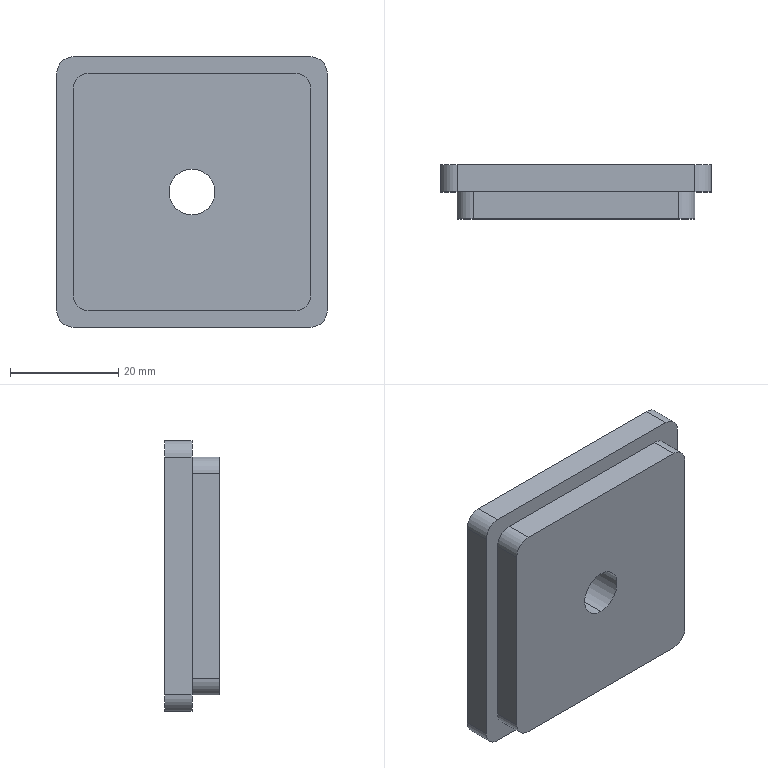Part | STEP file | Microwave Drying Flat Conveyor-CN2500x400-105-105 | 1 solid | 21 faces | box 50 x 10 x 50 mm | volume 21535 mm3 | plane 11 | cylinder 10 | commonest cylinder face diameters 6 x8 8.5 x2
STEP:
#1=CARTESIAN_POINT('',(0.,0.,-4.25));
#2=VERTEX_POINT('',#1);
#3=CARTESIAN_POINT('',(0.,0.,4.25));
#4=VERTEX_POINT('',#3);
#5=CARTESIAN_POINT('',(0.,0.,0.));
#6=DIRECTION('',(0.,1.,0.));
#7=DIRECTION('',(0.,0.,1.));
#8=AXIS2_PLACEMENT_3D('',#5,#6,#7);
#9=CIRCLE('',#8,4.25);
#10=EDGE_CURVE('',#2,#4,#9,.T.);
#11=ORIENTED_EDGE('',*,*,#10,.F.);
#12=CARTESIAN_POINT('',(0.,10.,-4.25));
#13=VERTEX_POINT('',#12);
#14=CARTESIAN_POINT('',(0.,10.,-4.25));
#15=DIRECTION('',(0.,1.,0.));
#16=VECTOR('',#15,1000.);
#17=LINE('',#14,#16);
#18=EDGE_CURVE('',#2,#13,#17,.T.);
#19=ORIENTED_EDGE('',*,*,#18,.T.);
#20=CARTESIAN_POINT('',(0.,10.,4.25));
#21=VERTEX_POINT('',#20);
#22=CARTESIAN_POINT('',(0.,10.,0.));
#23=DIRECTION('',(0.,1.,0.));
#24=DIRECTION('',(0.,0.,1.));
#25=AXIS2_PLACEMENT_3D('',#22,#23,#24);
#26=CIRCLE('',#25,4.25);
#27=EDGE_CURVE('',#13,#21,#26,.T.);
#28=ORIENTED_EDGE('',*,*,#27,.T.);
#29=CARTESIAN_POINT('',(0.,10.,4.25));
#30=DIRECTION('',(0.,1.,0.));
#31=VECTOR('',#30,1000.);
#32=LINE('',#29,#31);
#33=EDGE_CURVE('',#4,#21,#32,.T.);
#34=ORIENTED_EDGE('',*,*,#33,.F.);
#35=EDGE_LOOP('',(#11,#19,#28,#34));
#36=FACE_OUTER_BOUND('',#35,.T.);
#37=CARTESIAN_POINT('',(0.,10.,0.));
#38=DIRECTION('',(0.,1.,0.));
#39=DIRECTION('',(0.,0.,1.));
#40=AXIS2_PLACEMENT_3D('',#37,#38,#39);
#41=CYLINDRICAL_SURFACE('',#40,4.25);
#42=ADVANCED_FACE('',(#36),#41,.F.);
#43=CARTESIAN_POINT('',(25.,5.,22.));
#44=VERTEX_POINT('',#43);
#45=CARTESIAN_POINT('',(22.,5.,25.));
#46=VERTEX_POINT('',#45);
#47=CARTESIAN_POINT('',(22.,5.,22.));
#48=DIRECTION('',(0.,-1.,0.));
#49=DIRECTION('',(0.,0.,-1.));
#50=AXIS2_PLACEMENT_3D('',#47,#48,#49);
#51=CIRCLE('',#50,3.);
#52=EDGE_CURVE('',#44,#46,#51,.T.);
#53=ORIENTED_EDGE('',*,*,#52,.F.);
#54=CARTESIAN_POINT('',(25.,10.,22.));
#55=VERTEX_POINT('',#54);
#56=CARTESIAN_POINT('',(25.,10.,22.));
#57=DIRECTION('',(0.,-1.,0.));
#58=VECTOR('',#57,1000.);
#59=LINE('',#56,#58);
#60=EDGE_CURVE('',#55,#44,#59,.T.);
#61=ORIENTED_EDGE('',*,*,#60,.F.);
#62=CARTESIAN_POINT('',(22.,10.,25.));
#63=VERTEX_POINT('',#62);
#64=CARTESIAN_POINT('',(22.,10.,22.));
#65=DIRECTION('',(0.,1.,0.));
#66=DIRECTION('',(0.,0.,1.));
#67=AXIS2_PLACEMENT_3D('',#64,#65,#66);
#68=CIRCLE('',#67,3.);
#69=EDGE_CURVE('',#63,#55,#68,.T.);
#70=ORIENTED_EDGE('',*,*,#69,.F.);
#71=CARTESIAN_POINT('',(22.,10.,25.));
#72=DIRECTION('',(0.,-1.,0.));
#73=VECTOR('',#72,1000.);
#74=LINE('',#71,#73);
#75=EDGE_CURVE('',#63,#46,#74,.T.);
#76=ORIENTED_EDGE('',*,*,#75,.T.);
#77=EDGE_LOOP('',(#53,#61,#70,#76));
#78=FACE_OUTER_BOUND('',#77,.T.);
#79=CARTESIAN_POINT('',(22.,10.,22.));
#80=DIRECTION('',(0.,-1.,0.));
#81=DIRECTION('',(0.,0.,-1.));
#82=AXIS2_PLACEMENT_3D('',#79,#80,#81);
#83=CYLINDRICAL_SURFACE('',#82,3.);
#84=ADVANCED_FACE('',(#78),#83,.T.);
#85=CARTESIAN_POINT('',(25.,5.,-22.));
#86=VERTEX_POINT('',#85);
#87=CARTESIAN_POINT('',(25.,5.,22.));
#88=DIRECTION('',(0.,0.,1.));
#89=VECTOR('',#88,1000.);
#90=LINE('',#87,#89);
#91=EDGE_CURVE('',#86,#44,#90,.T.);
#92=ORIENTED_EDGE('',*,*,#91,.F.);
#93=CARTESIAN_POINT('',(25.,10.,-22.));
#94=VERTEX_POINT('',#93);
#95=CARTESIAN_POINT('',(25.,10.,-22.));
#96=DIRECTION('',(0.,-1.,0.));
#97=VECTOR('',#96,1000.);
#98=LINE('',#95,#97);
#99=EDGE_CURVE('',#94,#86,#98,.T.);
#100=ORIENTED_EDGE('',*,*,#99,.F.);
#101=CARTESIAN_POINT('',(25.,10.,-22.));
#102=DIRECTION('',(0.,0.,-1.));
#103=VECTOR('',#102,1000.);
#104=LINE('',#101,#103);
#105=EDGE_CURVE('',#55,#94,#104,.T.);
#106=ORIENTED_EDGE('',*,*,#105,.F.);
#107=ORIENTED_EDGE('',*,*,#60,.T.);
#108=EDGE_LOOP('',(#92,#100,#106,#107));
#109=FACE_OUTER_BOUND('',#108,.T.);
#110=CARTESIAN_POINT('',(25.,10.,-22.));
#111=DIRECTION('',(-1.,0.,0.));
#112=DIRECTION('',(0.,0.,1.));
#113=AXIS2_PLACEMENT_3D('',#110,#111,#112);
#114=PLANE('',#113);
#115=ADVANCED_FACE('',(#109),#114,.F.);
#116=CARTESIAN_POINT('',(22.,5.,-25.));
#117=VERTEX_POINT('',#116);
#118=CARTESIAN_POINT('',(22.,5.,-22.));
#119=DIRECTION('',(0.,-1.,0.));
#120=DIRECTION('',(0.,0.,-1.));
#121=AXIS2_PLACEMENT_3D('',#118,#119,#120);
#122=CIRCLE('',#121,3.);
#123=EDGE_CURVE('',#117,#86,#122,.T.);
#124=ORIENTED_EDGE('',*,*,#123,.F.);
#125=CARTESIAN_POINT('',(22.,10.,-25.));
#126=VERTEX_POINT('',#125);
#127=CARTESIAN_POINT('',(22.,10.,-25.));
#128=DIRECTION('',(0.,-1.,0.));
#129=VECTOR('',#128,1000.);
#130=LINE('',#127,#129);
#131=EDGE_CURVE('',#126,#117,#130,.T.);
#132=ORIENTED_EDGE('',*,*,#131,.F.);
#133=CARTESIAN_POINT('',(22.,10.,-22.));
#134=DIRECTION('',(0.,1.,0.));
#135=DIRECTION('',(0.,0.,-1.));
#136=AXIS2_PLACEMENT_3D('',#133,#134,#135);
#137=CIRCLE('',#136,3.);
#138=EDGE_CURVE('',#94,#126,#137,.T.);
#139=ORIENTED_EDGE('',*,*,#138,.F.);
#140=ORIENTED_EDGE('',*,*,#99,.T.);
#141=EDGE_LOOP('',(#124,#132,#139,#140));
#142=FACE_OUTER_BOUND('',#141,.T.);
#143=CARTESIAN_POINT('',(22.,10.,-22.));
#144=DIRECTION('',(0.,-1.,0.));
#145=DIRECTION('',(0.,0.,-1.));
#146=AXIS2_PLACEMENT_3D('',#143,#144,#145);
#147=CYLINDRICAL_SURFACE('',#146,3.);
#148=ADVANCED_FACE('',(#142),#147,.T.);
#149=CARTESIAN_POINT('',(-22.,5.,-25.));
#150=VERTEX_POINT('',#149);
#151=CARTESIAN_POINT('',(22.,5.,-25.));
#152=DIRECTION('',(1.,0.,0.));
#153=VECTOR('',#152,1000.);
#154=LINE('',#151,#153);
#155=EDGE_CURVE('',#150,#117,#154,.T.);
#156=ORIENTED_EDGE('',*,*,#155,.F.);
#157=CARTESIAN_POINT('',(-22.,10.,-25.));
#158=VERTEX_POINT('',#157);
#159=CARTESIAN_POINT('',(-22.,10.,-25.));
#160=DIRECTION('',(0.,-1.,0.));
#161=VECTOR('',#160,1000.);
#162=LINE('',#159,#161);
#163=EDGE_CURVE('',#158,#150,#162,.T.);
#164=ORIENTED_EDGE('',*,*,#163,.F.);
#165=CARTESIAN_POINT('',(-22.,10.,-25.));
#166=DIRECTION('',(-1.,0.,0.));
#167=VECTOR('',#166,1000.);
#168=LINE('',#165,#167);
#169=EDGE_CURVE('',#126,#158,#168,.T.);
#170=ORIENTED_EDGE('',*,*,#169,.F.);
#171=ORIENTED_EDGE('',*,*,#131,.T.);
#172=EDGE_LOOP('',(#156,#164,#170,#171));
#173=FACE_OUTER_BOUND('',#172,.T.);
#174=CARTESIAN_POINT('',(-22.,10.,-25.));
#175=DIRECTION('',(0.,0.,1.));
#176=DIRECTION('',(1.,0.,0.));
#177=AXIS2_PLACEMENT_3D('',#174,#175,#176);
#178=PLANE('',#177);
#179=ADVANCED_FACE('',(#173),#178,.F.);
#180=CARTESIAN_POINT('',(-25.,5.,-22.));
#181=VERTEX_POINT('',#180);
#182=CARTESIAN_POINT('',(-22.,5.,-22.));
#183=DIRECTION('',(0.,-1.,0.));
#184=DIRECTION('',(0.,0.,-1.));
#185=AXIS2_PLACEMENT_3D('',#182,#183,#184);
#186=CIRCLE('',#185,3.);
#187=EDGE_CURVE('',#181,#150,#186,.T.);
#188=ORIENTED_EDGE('',*,*,#187,.F.);
#189=CARTESIAN_POINT('',(-25.,10.,-22.));
#190=VERTEX_POINT('',#189);
#191=CARTESIAN_POINT('',(-25.,10.,-22.));
#192=DIRECTION('',(0.,-1.,0.));
#193=VECTOR('',#192,1000.);
#194=LINE('',#191,#193);
#195=EDGE_CURVE('',#190,#181,#194,.T.);
#196=ORIENTED_EDGE('',*,*,#195,.F.);
#197=CARTESIAN_POINT('',(-22.,10.,-22.));
#198=DIRECTION('',(0.,1.,0.));
#199=DIRECTION('',(0.,0.,1.));
#200=AXIS2_PLACEMENT_3D('',#197,#198,#199);
#201=CIRCLE('',#200,3.);
#202=EDGE_CURVE('',#158,#190,#201,.T.);
#203=ORIENTED_EDGE('',*,*,#202,.F.);
#204=ORIENTED_EDGE('',*,*,#163,.T.);
#205=EDGE_LOOP('',(#188,#196,#203,#204));
#206=FACE_OUTER_BOUND('',#205,.T.);
#207=CARTESIAN_POINT('',(-22.,10.,-22.));
#208=DIRECTION('',(0.,-1.,0.));
#209=DIRECTION('',(0.,0.,-1.));
#210=AXIS2_PLACEMENT_3D('',#207,#208,#209);
#211=CYLINDRICAL_SURFACE('',#210,3.);
#212=ADVANCED_FACE('',(#206),#211,.T.);
#213=CARTESIAN_POINT('',(-25.,5.,22.));
#214=VERTEX_POINT('',#213);
#215=CARTESIAN_POINT('',(-25.,5.,-22.));
#216=DIRECTION('',(0.,0.,-1.));
#217=VECTOR('',#216,1000.);
#218=LINE('',#215,#217);
#219=EDGE_CURVE('',#214,#181,#218,.T.);
#220=ORIENTED_EDGE('',*,*,#219,.F.);
#221=CARTESIAN_POINT('',(-25.,10.,22.));
#222=VERTEX_POINT('',#221);
#223=CARTESIAN_POINT('',(-25.,10.,22.));
#224=DIRECTION('',(0.,-1.,0.));
#225=VECTOR('',#224,1000.);
#226=LINE('',#223,#225);
#227=EDGE_CURVE('',#222,#214,#226,.T.);
#228=ORIENTED_EDGE('',*,*,#227,.F.);
#229=CARTESIAN_POINT('',(-25.,10.,-22.));
#230=DIRECTION('',(0.,0.,1.));
#231=VECTOR('',#230,1000.);
#232=LINE('',#229,#231);
#233=EDGE_CURVE('',#190,#222,#232,.T.);
#234=ORIENTED_EDGE('',*,*,#233,.F.);
#235=ORIENTED_EDGE('',*,*,#195,.T.);
#236=EDGE_LOOP('',(#220,#228,#234,#235));
#237=FACE_OUTER_BOUND('',#236,.T.);
#238=CARTESIAN_POINT('',(-25.,10.,-22.));
#239=DIRECTION('',(1.,0.,0.));
#240=DIRECTION('',(0.,0.,-1.));
#241=AXIS2_PLACEMENT_3D('',#238,#239,#240);
#242=PLANE('',#241);
#243=ADVANCED_FACE('',(#237),#242,.F.);
#244=CARTESIAN_POINT('',(-22.,5.,25.));
#245=VERTEX_POINT('',#244);
#246=CARTESIAN_POINT('',(-22.,5.,22.));
#247=DIRECTION('',(0.,-1.,0.));
#248=DIRECTION('',(0.,0.,-1.));
#249=AXIS2_PLACEMENT_3D('',#246,#247,#248);
#250=CIRCLE('',#249,3.);
#251=EDGE_CURVE('',#245,#214,#250,.T.);
#252=ORIENTED_EDGE('',*,*,#251,.F.);
#253=CARTESIAN_POINT('',(-22.,10.,25.));
#254=VERTEX_POINT('',#253);
#255=CARTESIAN_POINT('',(-22.,10.,25.));
#256=DIRECTION('',(0.,-1.,0.));
#257=VECTOR('',#256,1000.);
#258=LINE('',#255,#257);
#259=EDGE_CURVE('',#254,#245,#258,.T.);
#260=ORIENTED_EDGE('',*,*,#259,.F.);
#261=CARTESIAN_POINT('',(-22.,10.,22.));
#262=DIRECTION('',(0.,1.,0.));
#263=DIRECTION('',(0.,0.,1.));
#264=AXIS2_PLACEMENT_3D('',#261,#262,#263);
#265=CIRCLE('',#264,3.);
#266=EDGE_CURVE('',#222,#254,#265,.T.);
#267=ORIENTED_EDGE('',*,*,#266,.F.);
#268=ORIENTED_EDGE('',*,*,#227,.T.);
#269=EDGE_LOOP('',(#252,#260,#267,#268));
#270=FACE_OUTER_BOUND('',#269,.T.);
#271=CARTESIAN_POINT('',(-22.,10.,22.));
#272=DIRECTION('',(0.,-1.,0.));
#273=DIRECTION('',(0.,0.,-1.));
#274=AXIS2_PLACEMENT_3D('',#271,#272,#273);
#275=CYLINDRICAL_SURFACE('',#274,3.);
#276=ADVANCED_FACE('',(#270),#275,.T.);
#277=CARTESIAN_POINT('',(-22.,5.,25.));
#278=DIRECTION('',(-1.,0.,0.));
#279=VECTOR('',#278,1000.);
#280=LINE('',#277,#279);
#281=EDGE_CURVE('',#46,#245,#280,.T.);
#282=ORIENTED_EDGE('',*,*,#281,.F.);
#283=ORIENTED_EDGE('',*,*,#75,.F.);
#284=CARTESIAN_POINT('',(-22.,10.,25.));
#285=DIRECTION('',(1.,0.,0.));
#286=VECTOR('',#285,1000.);
#287=LINE('',#284,#286);
#288=EDGE_CURVE('',#254,#63,#287,.T.);
#289=ORIENTED_EDGE('',*,*,#288,.F.);
#290=ORIENTED_EDGE('',*,*,#259,.T.);
#291=EDGE_LOOP('',(#282,#283,#289,#290));
#292=FACE_OUTER_BOUND('',#291,.T.);
#293=CARTESIAN_POINT('',(-22.,10.,25.));
#294=DIRECTION('',(0.,0.,-1.));
#295=DIRECTION('',(-1.,0.,0.));
#296=AXIS2_PLACEMENT_3D('',#293,#294,#295);
#297=PLANE('',#296);
#298=ADVANCED_FACE('',(#292),#297,.F.);
#299=CARTESIAN_POINT('',(0.,0.,0.));
#300=DIRECTION('',(0.,1.,0.));
#301=DIRECTION('',(0.,0.,1.));
#302=AXIS2_PLACEMENT_3D('',#299,#300,#301);
#303=CIRCLE('',#302,4.25);
#304=EDGE_CURVE('',#4,#2,#303,.T.);
#305=ORIENTED_EDGE('',*,*,#304,.T.);
#306=ORIENTED_EDGE('',*,*,#10,.T.);
#307=EDGE_LOOP('',(#305,#306));
#308=FACE_BOUND('',#307,.T.);
#309=CARTESIAN_POINT('',(-22.,0.,19.));
#310=VERTEX_POINT('',#309);
#311=CARTESIAN_POINT('',(-22.,0.,-19.));
#312=VERTEX_POINT('',#311);
#313=CARTESIAN_POINT('',(-22.,0.,22.));
#314=DIRECTION('',(0.,0.,-1.));
#315=VECTOR('',#314,1000.);
#316=LINE('',#313,#315);
#317=EDGE_CURVE('',#310,#312,#316,.T.);
#318=ORIENTED_EDGE('',*,*,#317,.T.);
#319=CARTESIAN_POINT('',(-19.,0.,-22.));
#320=VERTEX_POINT('',#319);
#321=CARTESIAN_POINT('',(-19.,0.,-19.));
#322=DIRECTION('',(0.,-1.,0.));
#323=DIRECTION('',(0.,0.,1.));
#324=AXIS2_PLACEMENT_3D('',#321,#322,#323);
#325=CIRCLE('',#324,3.);
#326=EDGE_CURVE('',#312,#320,#325,.T.);
#327=ORIENTED_EDGE('',*,*,#326,.T.);
#328=CARTESIAN_POINT('',(19.,0.,-22.));
#329=VERTEX_POINT('',#328);
#330=CARTESIAN_POINT('',(-22.,0.,-22.));
#331=DIRECTION('',(1.,0.,0.));
#332=VECTOR('',#331,1000.);
#333=LINE('',#330,#332);
#334=EDGE_CURVE('',#320,#329,#333,.T.);
#335=ORIENTED_EDGE('',*,*,#334,.T.);
#336=CARTESIAN_POINT('',(22.,0.,-19.));
#337=VERTEX_POINT('',#336);
#338=CARTESIAN_POINT('',(19.,0.,-19.));
#339=DIRECTION('',(0.,-1.,0.));
#340=DIRECTION('',(0.,0.,1.));
#341=AXIS2_PLACEMENT_3D('',#338,#339,#340);
#342=CIRCLE('',#341,3.);
#343=EDGE_CURVE('',#329,#337,#342,.T.);
#344=ORIENTED_EDGE('',*,*,#343,.T.);
#345=CARTESIAN_POINT('',(22.,0.,19.));
#346=VERTEX_POINT('',#345);
#347=CARTESIAN_POINT('',(22.,0.,-22.));
#348=DIRECTION('',(0.,0.,1.));
#349=VECTOR('',#348,1000.);
#350=LINE('',#347,#349);
#351=EDGE_CURVE('',#337,#346,#350,.T.);
#352=ORIENTED_EDGE('',*,*,#351,.T.);
#353=CARTESIAN_POINT('',(19.,0.,22.));
#354=VERTEX_POINT('',#353);
#355=CARTESIAN_POINT('',(19.,0.,19.));
#356=DIRECTION('',(0.,-1.,0.));
#357=DIRECTION('',(0.,0.,1.));
#358=AXIS2_PLACEMENT_3D('',#355,#356,#357);
#359=CIRCLE('',#358,3.);
#360=EDGE_CURVE('',#346,#354,#359,.T.);
#361=ORIENTED_EDGE('',*,*,#360,.T.);
#362=CARTESIAN_POINT('',(-19.,0.,22.));
#363=VERTEX_POINT('',#362);
#364=CARTESIAN_POINT('',(22.,0.,22.));
#365=DIRECTION('',(-1.,0.,0.));
#366=VECTOR('',#365,1000.);
#367=LINE('',#364,#366);
#368=EDGE_CURVE('',#354,#363,#367,.T.);
#369=ORIENTED_EDGE('',*,*,#368,.T.);
#370=CARTESIAN_POINT('',(-19.,0.,19.));
#371=DIRECTION('',(0.,-1.,0.));
#372=DIRECTION('',(0.,0.,1.));
#373=AXIS2_PLACEMENT_3D('',#370,#371,#372);
#374=CIRCLE('',#373,3.);
#375=EDGE_CURVE('',#363,#310,#374,.T.);
#376=ORIENTED_EDGE('',*,*,#375,.T.);
#377=EDGE_LOOP('',(#318,#327,#335,#344,#352,#361,#369,#376));
#378=FACE_OUTER_BOUND('',#377,.T.);
#379=CARTESIAN_POINT('',(22.,0.,22.));
#380=DIRECTION('',(0.,1.,0.));
#381=DIRECTION('',(0.,0.,1.));
#382=AXIS2_PLACEMENT_3D('',#379,#380,#381);
#383=PLANE('',#382);
#384=ADVANCED_FACE('',(#308,#378),#383,.F.);
#385=CARTESIAN_POINT('',(0.,10.,0.));
#386=DIRECTION('',(0.,1.,0.));
#387=DIRECTION('',(0.,0.,1.));
#388=AXIS2_PLACEMENT_3D('',#385,#386,#387);
#389=CIRCLE('',#388,4.25);
#390=EDGE_CURVE('',#21,#13,#389,.T.);
#391=ORIENTED_EDGE('',*,*,#390,.F.);
#392=ORIENTED_EDGE('',*,*,#27,.F.);
#393=EDGE_LOOP('',(#391,#392));
#394=FACE_BOUND('',#393,.T.);
#395=ORIENTED_EDGE('',*,*,#69,.T.);
#396=ORIENTED_EDGE('',*,*,#105,.T.);
#397=ORIENTED_EDGE('',*,*,#138,.T.);
#398=ORIENTED_EDGE('',*,*,#169,.T.);
#399=ORIENTED_EDGE('',*,*,#202,.T.);
#400=ORIENTED_EDGE('',*,*,#233,.T.);
#401=ORIENTED_EDGE('',*,*,#266,.T.);
#402=ORIENTED_EDGE('',*,*,#288,.T.);
#403=EDGE_LOOP('',(#395,#396,#397,#398,#399,#400,#401,#402));
#404=FACE_OUTER_BOUND('',#403,.T.);
#405=CARTESIAN_POINT('',(22.,10.,22.));
#406=DIRECTION('',(0.,1.,0.));
#407=DIRECTION('',(0.,0.,1.));
#408=AXIS2_PLACEMENT_3D('',#405,#406,#407);
#409=PLANE('',#408);
#410=ADVANCED_FACE('',(#394,#404),#409,.T.);
#411=ORIENTED_EDGE('',*,*,#18,.F.);
#412=ORIENTED_EDGE('',*,*,#304,.F.);
#413=ORIENTED_EDGE('',*,*,#33,.T.);
#414=ORIENTED_EDGE('',*,*,#390,.T.);
#415=EDGE_LOOP('',(#411,#412,#413,#414));
#416=FACE_OUTER_BOUND('',#415,.T.);
#417=CARTESIAN_POINT('',(0.,10.,0.));
#418=DIRECTION('',(0.,1.,0.));
#419=DIRECTION('',(0.,0.,1.));
#420=AXIS2_PLACEMENT_3D('',#417,#418,#419);
#421=CYLINDRICAL_SURFACE('',#420,4.25);
#422=ADVANCED_FACE('',(#416),#421,.F.);
#423=CARTESIAN_POINT('',(-19.,5.,-22.));
#424=VERTEX_POINT('',#423);
#425=CARTESIAN_POINT('',(19.,5.,-22.));
#426=VERTEX_POINT('',#425);
#427=CARTESIAN_POINT('',(-22.,5.,-22.));
#428=DIRECTION('',(1.,0.,0.));
#429=VECTOR('',#428,1000.);
#430=LINE('',#427,#429);
#431=EDGE_CURVE('',#424,#426,#430,.T.);
#432=ORIENTED_EDGE('',*,*,#431,.F.);
#433=CARTESIAN_POINT('',(-22.,5.,-19.));
#434=VERTEX_POINT('',#433);
#435=CARTESIAN_POINT('',(-19.,5.,-19.));
#436=DIRECTION('',(0.,1.,0.));
#437=DIRECTION('',(0.,0.,-1.));
#438=AXIS2_PLACEMENT_3D('',#435,#436,#437);
#439=CIRCLE('',#438,3.);
#440=EDGE_CURVE('',#424,#434,#439,.T.);
#441=ORIENTED_EDGE('',*,*,#440,.T.);
#442=CARTESIAN_POINT('',(-22.,5.,19.));
#443=VERTEX_POINT('',#442);
#444=CARTESIAN_POINT('',(-22.,5.,22.));
#445=DIRECTION('',(0.,0.,-1.));
#446=VECTOR('',#445,1000.);
#447=LINE('',#444,#446);
#448=EDGE_CURVE('',#443,#434,#447,.T.);
#449=ORIENTED_EDGE('',*,*,#448,.F.);
#450=CARTESIAN_POINT('',(-19.,5.,22.));
#451=VERTEX_POINT('',#450);
#452=CARTESIAN_POINT('',(-19.,5.,19.));
#453=DIRECTION('',(0.,1.,0.));
#454=DIRECTION('',(0.,0.,-1.));
#455=AXIS2_PLACEMENT_3D('',#452,#453,#454);
#456=CIRCLE('',#455,3.);
#457=EDGE_CURVE('',#443,#451,#456,.T.);
#458=ORIENTED_EDGE('',*,*,#457,.T.);
#459=CARTESIAN_POINT('',(19.,5.,22.));
#460=VERTEX_POINT('',#459);
#461=CARTESIAN_POINT('',(22.,5.,22.));
#462=DIRECTION('',(-1.,0.,0.));
#463=VECTOR('',#462,1000.);
#464=LINE('',#461,#463);
#465=EDGE_CURVE('',#460,#451,#464,.T.);
#466=ORIENTED_EDGE('',*,*,#465,.F.);
#467=CARTESIAN_POINT('',(22.,5.,19.));
#468=VERTEX_POINT('',#467);
#469=CARTESIAN_POINT('',(19.,5.,19.));
#470=DIRECTION('',(0.,1.,0.));
#471=DIRECTION('',(0.,0.,-1.));
#472=AXIS2_PLACEMENT_3D('',#469,#470,#471);
#473=CIRCLE('',#472,3.);
#474=EDGE_CURVE('',#460,#468,#473,.T.);
#475=ORIENTED_EDGE('',*,*,#474,.T.);
#476=CARTESIAN_POINT('',(22.,5.,-19.));
#477=VERTEX_POINT('',#476);
#478=CARTESIAN_POINT('',(22.,5.,-22.));
#479=DIRECTION('',(0.,0.,1.));
#480=VECTOR('',#479,1000.);
#481=LINE('',#478,#480);
#482=EDGE_CURVE('',#477,#468,#481,.T.);
#483=ORIENTED_EDGE('',*,*,#482,.F.);
#484=CARTESIAN_POINT('',(19.,5.,-19.));
#485=DIRECTION('',(0.,1.,0.));
#486=DIRECTION('',(0.,0.,-1.));
#487=AXIS2_PLACEMENT_3D('',#484,#485,#486);
#488=CIRCLE('',#487,3.);
#489=EDGE_CURVE('',#477,#426,#488,.T.);
#490=ORIENTED_EDGE('',*,*,#489,.T.);
#491=EDGE_LOOP('',(#432,#441,#449,#458,#466,#475,#483,#490));
#492=FACE_BOUND('',#491,.T.);
#493=ORIENTED_EDGE('',*,*,#251,.T.);
#494=ORIENTED_EDGE('',*,*,#219,.T.);
#495=ORIENTED_EDGE('',*,*,#187,.T.);
#496=ORIENTED_EDGE('',*,*,#155,.T.);
#497=ORIENTED_EDGE('',*,*,#123,.T.);
#498=ORIENTED_EDGE('',*,*,#91,.T.);
#499=ORIENTED_EDGE('',*,*,#52,.T.);
#500=ORIENTED_EDGE('',*,*,#281,.T.);
#501=EDGE_LOOP('',(#493,#494,#495,#496,#497,#498,#499,#500));
#502=FACE_OUTER_BOUND('',#501,.T.);
#503=CARTESIAN_POINT('',(-22.,5.,22.));
#504=DIRECTION('',(0.,-1.,0.));
#505=DIRECTION('',(0.,0.,-1.));
#506=AXIS2_PLACEMENT_3D('',#503,#504,#505);
#507=PLANE('',#506);
#508=ADVANCED_FACE('',(#492,#502),#507,.T.);
#509=ORIENTED_EDGE('',*,*,#482,.T.);
#510=CARTESIAN_POINT('',(22.,5.,19.));
#511=DIRECTION('',(0.,-1.,0.));
#512=VECTOR('',#511,1000.);
#513=LINE('',#510,#512);
#514=EDGE_CURVE('',#468,#346,#513,.T.);
#515=ORIENTED_EDGE('',*,*,#514,.T.);
#516=ORIENTED_EDGE('',*,*,#351,.F.);
#517=CARTESIAN_POINT('',(22.,5.,-19.));
#518=DIRECTION('',(0.,1.,0.));
#519=VECTOR('',#518,1000.);
#520=LINE('',#517,#519);
#521=EDGE_CURVE('',#337,#477,#520,.T.);
#522=ORIENTED_EDGE('',*,*,#521,.T.);
#523=EDGE_LOOP('',(#509,#515,#516,#522));
#524=FACE_OUTER_BOUND('',#523,.T.);
#525=CARTESIAN_POINT('',(22.,5.,-22.));
#526=DIRECTION('',(1.,0.,0.));
#527=DIRECTION('',(0.,0.,-1.));
#528=AXIS2_PLACEMENT_3D('',#525,#526,#527);
#529=PLANE('',#528);
#530=ADVANCED_FACE('',(#524),#529,.T.);
#531=ORIENTED_EDGE('',*,*,#334,.F.);
#532=CARTESIAN_POINT('',(-19.,5.,-22.));
#533=DIRECTION('',(0.,1.,0.));
#534=VECTOR('',#533,1000.);
#535=LINE('',#532,#534);
#536=EDGE_CURVE('',#320,#424,#535,.T.);
#537=ORIENTED_EDGE('',*,*,#536,.T.);
#538=ORIENTED_EDGE('',*,*,#431,.T.);
#539=CARTESIAN_POINT('',(19.,5.,-22.));
#540=DIRECTION('',(0.,-1.,0.));
#541=VECTOR('',#540,1000.);
#542=LINE('',#539,#541);
#543=EDGE_CURVE('',#426,#329,#542,.T.);
#544=ORIENTED_EDGE('',*,*,#543,.T.);
#545=EDGE_LOOP('',(#531,#537,#538,#544));
#546=FACE_OUTER_BOUND('',#545,.T.);
#547=CARTESIAN_POINT('',(-22.,5.,-22.));
#548=DIRECTION('',(0.,0.,-1.));
#549=DIRECTION('',(-1.,0.,0.));
#550=AXIS2_PLACEMENT_3D('',#547,#548,#549);
#551=PLANE('',#550);
#552=ADVANCED_FACE('',(#546),#551,.T.);
#553=ORIENTED_EDGE('',*,*,#448,.T.);
#554=CARTESIAN_POINT('',(-22.,5.,-19.));
#555=DIRECTION('',(0.,-1.,0.));
#556=VECTOR('',#555,1000.);
#557=LINE('',#554,#556);
#558=EDGE_CURVE('',#434,#312,#557,.T.);
#559=ORIENTED_EDGE('',*,*,#558,.T.);
#560=ORIENTED_EDGE('',*,*,#317,.F.);
#561=CARTESIAN_POINT('',(-22.,5.,19.));
#562=DIRECTION('',(0.,1.,0.));
#563=VECTOR('',#562,1000.);
#564=LINE('',#561,#563);
#565=EDGE_CURVE('',#310,#443,#564,.T.);
#566=ORIENTED_EDGE('',*,*,#565,.T.);
#567=EDGE_LOOP('',(#553,#559,#560,#566));
#568=FACE_OUTER_BOUND('',#567,.T.);
#569=CARTESIAN_POINT('',(-22.,5.,22.));
#570=DIRECTION('',(-1.,0.,0.));
#571=DIRECTION('',(0.,0.,1.));
#572=AXIS2_PLACEMENT_3D('',#569,#570,#571);
#573=PLANE('',#572);
#574=ADVANCED_FACE('',(#568),#573,.T.);
#575=ORIENTED_EDGE('',*,*,#465,.T.);
#576=CARTESIAN_POINT('',(-19.,5.,22.));
#577=DIRECTION('',(0.,-1.,0.));
#578=VECTOR('',#577,1000.);
#579=LINE('',#576,#578);
#580=EDGE_CURVE('',#451,#363,#579,.T.);
#581=ORIENTED_EDGE('',*,*,#580,.T.);
#582=ORIENTED_EDGE('',*,*,#368,.F.);
#583=CARTESIAN_POINT('',(19.,5.,22.));
#584=DIRECTION('',(0.,1.,0.));
#585=VECTOR('',#584,1000.);
#586=LINE('',#583,#585);
#587=EDGE_CURVE('',#354,#460,#586,.T.);
#588=ORIENTED_EDGE('',*,*,#587,.T.);
#589=EDGE_LOOP('',(#575,#581,#582,#588));
#590=FACE_OUTER_BOUND('',#589,.T.);
#591=CARTESIAN_POINT('',(22.,5.,22.));
#592=DIRECTION('',(0.,0.,1.));
#593=DIRECTION('',(1.,0.,0.));
#594=AXIS2_PLACEMENT_3D('',#591,#592,#593);
#595=PLANE('',#594);
#596=ADVANCED_FACE('',(#590),#595,.T.);
#597=ORIENTED_EDGE('',*,*,#440,.F.);
#598=ORIENTED_EDGE('',*,*,#536,.F.);
#599=ORIENTED_EDGE('',*,*,#326,.F.);
#600=ORIENTED_EDGE('',*,*,#558,.F.);
#601=EDGE_LOOP('',(#597,#598,#599,#600));
#602=FACE_OUTER_BOUND('',#601,.T.);
#603=CARTESIAN_POINT('',(-19.,5.,-19.));
#604=DIRECTION('',(0.,-1.,0.));
#605=DIRECTION('',(0.,0.,-1.));
#606=AXIS2_PLACEMENT_3D('',#603,#604,#605);
#607=CYLINDRICAL_SURFACE('',#606,3.);
#608=ADVANCED_FACE('',(#602),#607,.T.);
#609=ORIENTED_EDGE('',*,*,#457,.F.);
#610=ORIENTED_EDGE('',*,*,#565,.F.);
#611=ORIENTED_EDGE('',*,*,#375,.F.);
#612=ORIENTED_EDGE('',*,*,#580,.F.);
#613=EDGE_LOOP('',(#609,#610,#611,#612));
#614=FACE_OUTER_BOUND('',#613,.T.);
#615=CARTESIAN_POINT('',(-19.,5.,19.));
#616=DIRECTION('',(0.,-1.,0.));
#617=DIRECTION('',(0.,0.,-1.));
#618=AXIS2_PLACEMENT_3D('',#615,#616,#617);
#619=CYLINDRICAL_SURFACE('',#618,3.);
#620=ADVANCED_FACE('',(#614),#619,.T.);
#621=ORIENTED_EDGE('',*,*,#474,.F.);
#622=ORIENTED_EDGE('',*,*,#587,.F.);
#623=ORIENTED_EDGE('',*,*,#360,.F.);
#624=ORIENTED_EDGE('',*,*,#514,.F.);
#625=EDGE_LOOP('',(#621,#622,#623,#624));
#626=FACE_OUTER_BOUND('',#625,.T.);
#627=CARTESIAN_POINT('',(19.,5.,19.));
#628=DIRECTION('',(0.,-1.,0.));
#629=DIRECTION('',(0.,0.,-1.));
#630=AXIS2_PLACEMENT_3D('',#627,#628,#629);
#631=CYLINDRICAL_SURFACE('',#630,3.);
#632=ADVANCED_FACE('',(#626),#631,.T.);
#633=ORIENTED_EDGE('',*,*,#489,.F.);
#634=ORIENTED_EDGE('',*,*,#521,.F.);
#635=ORIENTED_EDGE('',*,*,#343,.F.);
#636=ORIENTED_EDGE('',*,*,#543,.F.);
#637=EDGE_LOOP('',(#633,#634,#635,#636));
#638=FACE_OUTER_BOUND('',#637,.T.);
#639=CARTESIAN_POINT('',(19.,5.,-19.));
#640=DIRECTION('',(0.,-1.,0.));
#641=DIRECTION('',(0.,0.,-1.));
#642=AXIS2_PLACEMENT_3D('',#639,#640,#641);
#643=CYLINDRICAL_SURFACE('',#642,3.);
#644=ADVANCED_FACE('',(#638),#643,.T.);
#645=CLOSED_SHELL('',(#42,#84,#115,#148,#179,#212,#243,#276,#298,#384,#410,#422,#508,#530,#552,#574,#596,#608,#620,#632,#644));
#646=MANIFOLD_SOLID_BREP('',#645);
#647=CARTESIAN_POINT('',(0.,0.,0.));
#648=DIRECTION('',(0.,0.,1.));
#649=DIRECTION('',(1.,0.,0.));
#650=AXIS2_PLACEMENT_3D('',#647,#648,#649);
#651=(LENGTH_UNIT()NAMED_UNIT(*)SI_UNIT(.MILLI.,.METRE.));
#652=UNCERTAINTY_MEASURE_WITH_UNIT(LENGTH_MEASURE(0.00001),#651,'','');
#653=(NAMED_UNIT(*)PLANE_ANGLE_UNIT()SI_UNIT($,.RADIAN.));
#654=(NAMED_UNIT(*)SI_UNIT($,.STERADIAN.)SOLID_ANGLE_UNIT());
#655=(GEOMETRIC_REPRESENTATION_CONTEXT(3)GLOBAL_UNCERTAINTY_ASSIGNED_CONTEXT((#652))GLOBAL_UNIT_ASSIGNED_CONTEXT((#651,#653,#654))REPRESENTATION_CONTEXT('',''));
#656=ADVANCED_BREP_SHAPE_REPRESENTATION('',(#646,#650),#655);